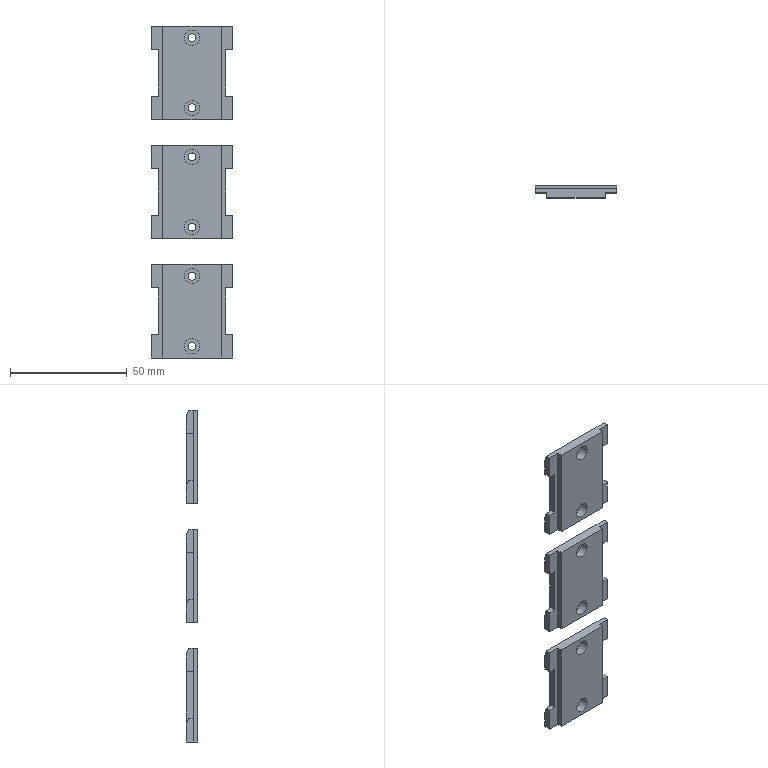CAM job | NX | 3+2 milling, drilling | part box 35 x 5 x 142 mm | stock box 40 x 8 x 147 mm
Tools:
number,name,description,diameter,corner_radius,flute_length,length,flutes
4,D4,平底铣刀-粗,4.0,0.0,25.0,75.0,2
6,D6,平底铣刀-粗,6.0,0.0,25.0,75.0,2
9,D10,平底铣刀-粗,10.0,0.0,35.0,75.0,2
17,D2-J,平底铣刀-精,2.0,0.0,50.0,75.0,2
11,D4-J,平底铣刀-精,4.0,0.0,50.0,75.0,2
7,D6-J,平底铣刀-精,6.0,0.0,25.0,75.0,2
10,D10-J,平底铣刀-精,10.0,0.0,35.0,75.0,2
17,D6R0.5-J,圆鼻刀-精,6.0,0.5,50.0,75.0,2
2,D6_CHAMFER_TOOL,倒角刀,6.0,0.0,3.0,25.0,2
13,ZT3.4,钻头,3.4,0.0,35.0,50.0,2
Operations:
program,operation,operation_type,tool,method,geometry_group,spindle_rpm,surface_speed,feed_per_tooth,feed_cut,feed_plunge,cut_length_mm,path_length_mm,cut_time_min,machine_time_min
D,等高往复层切开粗-中_COPY_COPY,ZLevelMilling,D6,分层开粗-切深K-步距G,W-D,8000.0,150.796,0.1875,3000.0,100.0,147.001,387.444,0.049,0.073
D,底壁铣精光底面-中_COPY_COPY,VolumeBased25DMillingOperation,D6-J,精光步距切深关,W-D,7000.0,175.0,0.0536,1500.0,100.0,46.34,74.34,0.0309,0.0337
D,底壁铣精光侧面-中-选底面_COPY_COPY,VolumeBased25DMillingOperation,D6-J,侧刃精光-切深K-步距G,W-D,8000.0,251.32,0.0625,1000.0,100.0,33.641,73.841,0.0336,0.0377
D,平面去毛刺6X45L_COPY_COPY,SurfaceContour,D6_CHAMFER_TOOL,爬面_倒角-切深0-步距G,W-D,6500.0,122.519,0.1154,1500.0,100.0,70.221,220.304,0.0468,0.0618
C,等高往复层切开粗-中_COPY,ZLevelMilling,D6,分层开粗-切深K-步距G,W-C,8000.0,150.796,0.1875,3000.0,100.0,147.001,375.911,0.049,0.0719
C,底壁铣精光底面-中_COPY,VolumeBased25DMillingOperation,D6-J,精光步距切深关,W-C,7000.0,175.0,0.0536,1500.0,100.0,46.34,70.14,0.0309,0.0333
C,底壁铣精光侧面-中-选底面_COPY,VolumeBased25DMillingOperation,D6-J,侧刃精光-切深K-步距G,W-C,8000.0,251.32,0.0625,1000.0,100.0,33.641,68.864,0.0336,0.0372
C,平面去毛刺6X45L_COPY,SurfaceContour,D6_CHAMFER_TOOL,爬面_倒角-切深0-步距G,W-C,6500.0,122.519,0.1154,1500.0,100.0,70.221,220.304,0.0468,0.0618
B,面铣自动飞面精光_COPY_COPY,FaceMilling,D6-J,侧刃精光-切深K-步距G,W-B,8000.0,251.327,0.0625,1000.0,100.0,8338.072,9068.31,8.338,8.411
B,面铣自动飞面精光_COPY_COPY_COPY,FaceMilling,D6-J,侧刃精光-切深K-步距G,W-B,8000.0,251.327,0.0625,1000.0,100.0,1667.614,1723.614,1.668,1.673
B,等高精光往复爬面_COPY,ZLevelMilling,D6R0.5-J,等高爬面-切深K-步距G,W-B,10000.0,188.496,0.175,3500.0,100.0,4577.976,4800.555,1.308,1.33
B,C0.3封闭铣廓倒角6X45L_COPY,PlanarMilling,D6_CHAMFER_TOOL,爬面_倒角-切深0-步距G,W-B,7000.0,131.0,0.1071,1500.0,100.0,534.599,786.566,0.3564,0.3816
B,NG_钻倒角_1,Operation,D6_CHAMFER_TOOL,METHOD,W-B,8000.0,150.796,0.0625,1000.0,0.0,30.0,267.875,0.03,0.0538
A,面铣自动飞面精光_COPY,FaceMilling,D10-J,侧刃精光-切深K-步距G,W-A,8000.0,251.327,0.0625,1000.0,100.0,1193.877,1249.877,1.194,1.2
A,外形粗_2,VolumeBased25DMillingOperation,D10,METHOD,W-A,6000.0,188.0,0.25,4000.0,80.0,7291.306,7634.61,1.823,1.857
A,沉头孔打点-深0.8,Operation,D6_CHAMFER_TOOL,NONE,W-A,8000.0,150.796,0.0312,500.0,90.0,10.8,218.698,0.0216,0.0424
A,沉头孔-钻孔0段,Operation,ZT3.4,NONE,W-A,2800.0,29.908,0.0179,100.0,90.0,54.129,305.355,0.5413,0.5664
A,底壁粗_1,VolumeBased25DMillingOperation,D4,METHOD,W-A,9000.0,113.097,0.1111,2000.0,100.0,4814.4,5611.113,2.407,2.487
A,铣孔开粗D4_1,CylinderMilling,D4,NONE,W-A,8000.0,100.531,0.075,1200.0,100.0,629.118,1138.518,0.5243,0.5752
A,铣孔精光D4_1,CylinderMilling,D4-J,精光步距切深关,W-A,8000.0,100.531,0.0312,500.0,100.0,113.737,623.137,0.2275,0.2784
A,外形D4清角,ZLevelMilling,D2-J,METHOD,W-A,6000.0,75.0,0.25,2500.0,80.0,1470.609,2233.05,0.5901,0.6663
A,CHAMFER_2,SurfaceContour,D6_CHAMFER_TOOL,METHOD,W-A,6000.0,113.0,0.125,1200.0,100.0,787.591,2135.097,0.6563,0.7911
A,铣倒角_1,PlanarMilling,D6_CHAMFER_TOOL,NONE,W-A,8000.0,150.796,0.0312,500.0,100.0,175.533,666.437,0.3511,0.4002
A,底精_1,VolumeBased25DMillingOperation,D4-J,METHOD,W-A,8000.0,100.531,0.075,1200.0,100.0,627.0,1224.01,0.5225,0.5822
A,底侧精_3,VolumeBased25DMillingOperation,D4-J,METHOD,W-A,8000.0,100.531,0.075,1200.0,100.0,287.65,861.19,0.2397,0.2971
A,外形精_2,VolumeBased25DMillingOperation,D4-J,METHOD,W-A,6000.0,113.0,0.0833,1000.0,100.0,527.421,889.234,0.5274,0.5636
E,等高光顺清角D2参考6_COPY,ZLevelMilling,D2-J,分层精光-切深K-步距G,W-B,8000.0,50.266,0.075,1200.0,100.0,7791.633,8471.124,6.493,6.561